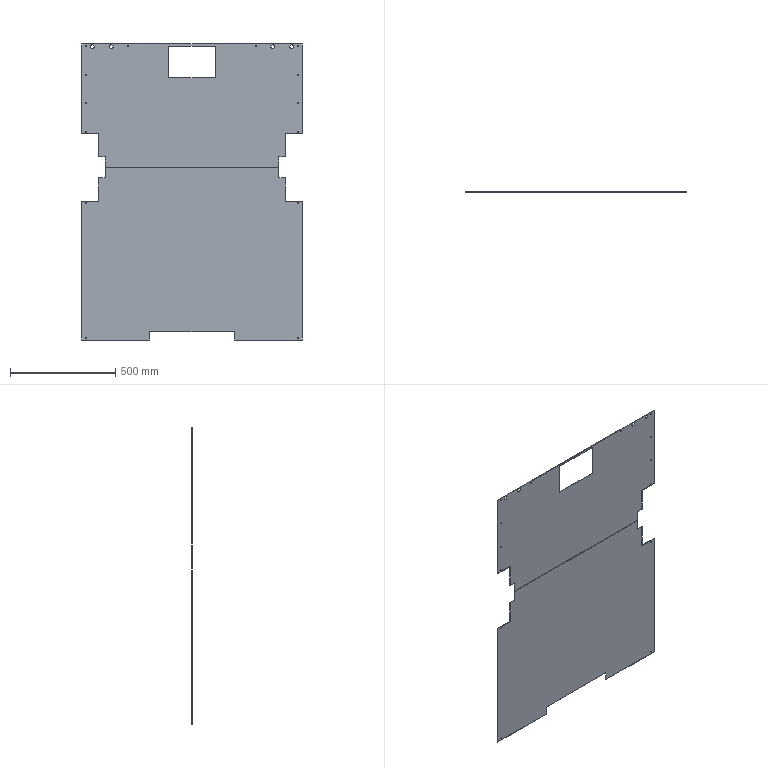Part | SolidWorks | features ICE 10, FlatPattern 2, SMBaseFlange 1, SheetMetal 1 | 2 solids | 72 faces | box 1050 x 1 x 1406 mm | volume 1366400 mm3 | cylinder 36 | plane 36 | commonest cylinder face diameters 5 x28 18 x8